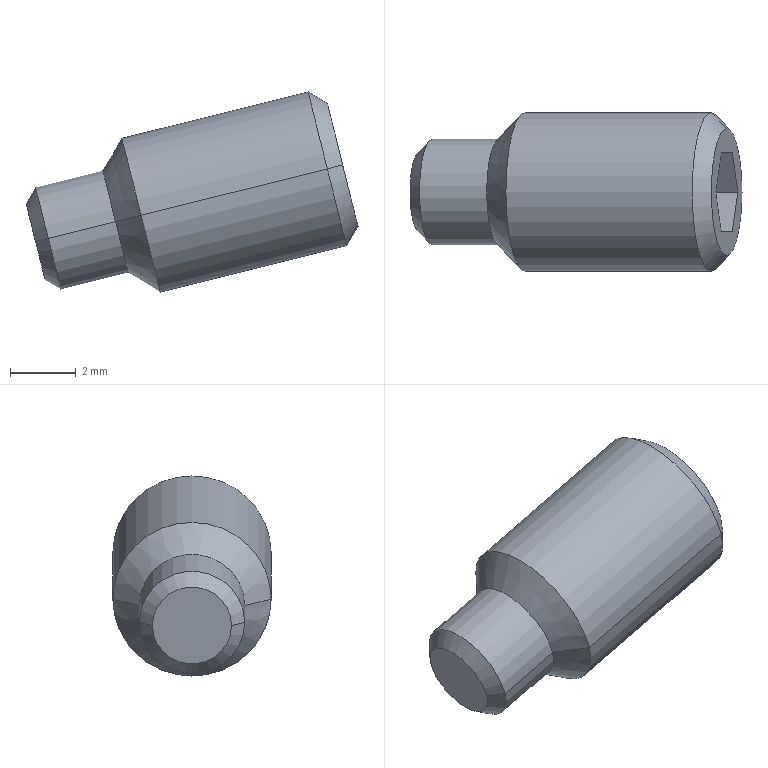Part | SolidWorks | features BaseBody 1 | 1 solid | 19 faces | box 10.07 x 4.8 x 6.065 mm | volume 127.97 mm3 | plane 9 | cone 6 | cylinder 4 | commonest cylinder face diameters 3.2 x2 4.8 x2
STEP:
#1=CARTESIAN_POINT('',(-2069.33,548.067,-1553.025));
#2=VERTEX_POINT('',#1);
#3=CARTESIAN_POINT('',(-2069.718,548.467,-1553.121));
#4=VERTEX_POINT('',#3);
#5=CARTESIAN_POINT('',(-2069.33,548.067,-1553.025));
#6=DIRECTION('',(-0.6861,0.7071,-0.1711));
#7=VECTOR('',#6,1000.);
#8=LINE('',#5,#7);
#9=EDGE_CURVE('',#2,#4,#8,.T.);
#10=ORIENTED_EDGE('',*,*,#9,.T.);
#11=CARTESIAN_POINT('',(-2069.718,550.867,-1553.121));
#12=VERTEX_POINT('',#11);
#13=CARTESIAN_POINT('',(-2069.718,549.667,-1553.121));
#14=DIRECTION('',(-0.9703,0.,-0.2419));
#15=DIRECTION('',(0.,1.,0.));
#16=AXIS2_PLACEMENT_3D('',#13,#14,#15);
#17=CIRCLE('',#16,1.2);
#18=EDGE_CURVE('',#12,#4,#17,.T.);
#19=ORIENTED_EDGE('',*,*,#18,.F.);
#20=CARTESIAN_POINT('',(-2069.33,551.267,-1553.025));
#21=VERTEX_POINT('',#20);
#22=CARTESIAN_POINT('',(-2069.718,550.867,-1553.121));
#23=DIRECTION('',(0.6861,0.7071,0.1711));
#24=VECTOR('',#23,1000.);
#25=LINE('',#22,#24);
#26=EDGE_CURVE('',#12,#21,#25,.T.);
#27=ORIENTED_EDGE('',*,*,#26,.T.);
#28=CARTESIAN_POINT('',(-2069.33,549.667,-1553.025));
#29=DIRECTION('',(0.9703,0.,0.2419));
#30=DIRECTION('',(0.,-1.,0.));
#31=AXIS2_PLACEMENT_3D('',#28,#29,#30);
#32=CIRCLE('',#31,1.6);
#33=EDGE_CURVE('',#2,#21,#32,.T.);
#34=ORIENTED_EDGE('',*,*,#33,.F.);
#35=EDGE_LOOP('',(#10,#19,#27,#34));
#36=FACE_OUTER_BOUND('',#35,.T.);
#37=CARTESIAN_POINT('',(-2069.738,549.667,-1553.126));
#38=DIRECTION('',(0.9703,0.,0.2419));
#39=DIRECTION('',(-0.02108,-0.9962,0.08457));
#40=AXIS2_PLACEMENT_3D('',#37,#38,#39);
#41=CONICAL_SURFACE('',#40,1.18,0.7854);
#42=ADVANCED_FACE('',(#36),#41,.T.);
#43=CARTESIAN_POINT('',(-2067.293,548.067,-1552.517));
#44=VERTEX_POINT('',#43);
#45=CARTESIAN_POINT('',(-2067.293,548.067,-1552.517));
#46=DIRECTION('',(-0.9703,0.,-0.2419));
#47=VECTOR('',#46,1000.);
#48=LINE('',#45,#47);
#49=EDGE_CURVE('',#44,#2,#48,.T.);
#50=ORIENTED_EDGE('',*,*,#49,.T.);
#51=ORIENTED_EDGE('',*,*,#33,.T.);
#52=CARTESIAN_POINT('',(-2067.293,551.267,-1552.517));
#53=VERTEX_POINT('',#52);
#54=CARTESIAN_POINT('',(-2069.33,551.267,-1553.025));
#55=DIRECTION('',(0.9703,0.,0.2419));
#56=VECTOR('',#55,1000.);
#57=LINE('',#54,#56);
#58=EDGE_CURVE('',#21,#53,#57,.T.);
#59=ORIENTED_EDGE('',*,*,#58,.T.);
#60=CARTESIAN_POINT('',(-2067.293,549.667,-1552.517));
#61=DIRECTION('',(0.9703,0.,0.2419));
#62=DIRECTION('',(0.,-1.,0.));
#63=AXIS2_PLACEMENT_3D('',#60,#61,#62);
#64=CIRCLE('',#63,1.6);
#65=EDGE_CURVE('',#44,#53,#64,.T.);
#66=ORIENTED_EDGE('',*,*,#65,.F.);
#67=EDGE_LOOP('',(#50,#51,#59,#66));
#68=FACE_OUTER_BOUND('',#67,.T.);
#69=CARTESIAN_POINT('',(-2067.191,549.667,-1552.491));
#70=DIRECTION('',(0.9703,0.,0.2419));
#71=DIRECTION('',(-0.02108,-0.9962,0.08457));
#72=AXIS2_PLACEMENT_3D('',#69,#70,#71);
#73=CYLINDRICAL_SURFACE('',#72,1.6);
#74=ADVANCED_FACE('',(#68),#73,.T.);
#75=CARTESIAN_POINT('',(-2066.517,547.267,-1552.323));
#76=VERTEX_POINT('',#75);
#77=CARTESIAN_POINT('',(-2066.517,547.267,-1552.323));
#78=DIRECTION('',(-0.6861,0.7071,-0.1711));
#79=VECTOR('',#78,1000.);
#80=LINE('',#77,#79);
#81=EDGE_CURVE('',#76,#44,#80,.T.);
#82=ORIENTED_EDGE('',*,*,#81,.T.);
#83=ORIENTED_EDGE('',*,*,#65,.T.);
#84=CARTESIAN_POINT('',(-2066.517,552.067,-1552.323));
#85=VERTEX_POINT('',#84);
#86=CARTESIAN_POINT('',(-2067.293,551.267,-1552.517));
#87=DIRECTION('',(0.6861,0.7071,0.1711));
#88=VECTOR('',#87,1000.);
#89=LINE('',#86,#88);
#90=EDGE_CURVE('',#53,#85,#89,.T.);
#91=ORIENTED_EDGE('',*,*,#90,.T.);
#92=CARTESIAN_POINT('',(-2066.517,549.667,-1552.323));
#93=DIRECTION('',(0.9703,0.,0.2419));
#94=DIRECTION('',(0.,-1.,0.));
#95=AXIS2_PLACEMENT_3D('',#92,#93,#94);
#96=CIRCLE('',#95,2.4);
#97=EDGE_CURVE('',#76,#85,#96,.T.);
#98=ORIENTED_EDGE('',*,*,#97,.F.);
#99=EDGE_LOOP('',(#82,#83,#91,#98));
#100=FACE_OUTER_BOUND('',#99,.T.);
#101=CARTESIAN_POINT('',(-2067.332,549.667,-1552.526));
#102=DIRECTION('',(0.9703,0.,0.2419));
#103=DIRECTION('',(-0.02108,-0.9962,0.08457));
#104=AXIS2_PLACEMENT_3D('',#101,#102,#103);
#105=CONICAL_SURFACE('',#104,1.56,0.7854);
#106=ADVANCED_FACE('',(#100),#105,.T.);
#107=CARTESIAN_POINT('',(-2060.869,547.267,-1550.915));
#108=VERTEX_POINT('',#107);
#109=CARTESIAN_POINT('',(-2060.404,547.747,-1550.799));
#110=VERTEX_POINT('',#109);
#111=CARTESIAN_POINT('',(-2060.869,547.267,-1550.915));
#112=DIRECTION('',(0.6861,0.7071,0.1711));
#113=VECTOR('',#112,1000.);
#114=LINE('',#111,#113);
#115=EDGE_CURVE('',#108,#110,#114,.T.);
#116=ORIENTED_EDGE('',*,*,#115,.T.);
#117=CARTESIAN_POINT('',(-2060.404,551.587,-1550.799));
#118=VERTEX_POINT('',#117);
#119=CARTESIAN_POINT('',(-2060.404,549.667,-1550.799));
#120=DIRECTION('',(0.9703,0.,0.2419));
#121=DIRECTION('',(0.,1.,0.));
#122=AXIS2_PLACEMENT_3D('',#119,#120,#121);
#123=CIRCLE('',#122,1.92);
#124=EDGE_CURVE('',#118,#110,#123,.T.);
#125=ORIENTED_EDGE('',*,*,#124,.F.);
#126=CARTESIAN_POINT('',(-2060.869,552.067,-1550.915));
#127=VERTEX_POINT('',#126);
#128=CARTESIAN_POINT('',(-2060.404,551.587,-1550.799));
#129=DIRECTION('',(-0.6861,0.7071,-0.1711));
#130=VECTOR('',#129,1000.);
#131=LINE('',#128,#130);
#132=EDGE_CURVE('',#118,#127,#131,.T.);
#133=ORIENTED_EDGE('',*,*,#132,.T.);
#134=CARTESIAN_POINT('',(-2060.869,549.667,-1550.915));
#135=DIRECTION('',(-0.9703,0.,-0.2419));
#136=DIRECTION('',(0.,-1.,0.));
#137=AXIS2_PLACEMENT_3D('',#134,#135,#136);
#138=CIRCLE('',#137,2.4);
#139=EDGE_CURVE('',#108,#127,#138,.T.);
#140=ORIENTED_EDGE('',*,*,#139,.F.);
#141=EDGE_LOOP('',(#116,#125,#133,#140));
#142=FACE_OUTER_BOUND('',#141,.T.);
#143=CARTESIAN_POINT('',(-2060.38,549.667,-1550.793));
#144=DIRECTION('',(-0.9703,0.,-0.2419));
#145=DIRECTION('',(0.02108,-0.9962,-0.08457));
#146=AXIS2_PLACEMENT_3D('',#143,#144,#145);
#147=CONICAL_SURFACE('',#146,1.896,0.7854);
#148=ADVANCED_FACE('',(#142),#147,.T.);
#149=CARTESIAN_POINT('',(-2066.517,552.067,-1552.323));
#150=DIRECTION('',(0.9703,0.,0.2419));
#151=VECTOR('',#150,1000.);
#152=LINE('',#149,#151);
#153=EDGE_CURVE('',#85,#127,#152,.T.);
#154=ORIENTED_EDGE('',*,*,#153,.T.);
#155=CARTESIAN_POINT('',(-2060.869,549.667,-1550.915));
#156=DIRECTION('',(-0.9703,0.,-0.2419));
#157=DIRECTION('',(0.,1.,0.));
#158=AXIS2_PLACEMENT_3D('',#155,#156,#157);
#159=CIRCLE('',#158,2.4);
#160=EDGE_CURVE('',#127,#108,#159,.T.);
#161=ORIENTED_EDGE('',*,*,#160,.T.);
#162=CARTESIAN_POINT('',(-2060.869,547.267,-1550.915));
#163=DIRECTION('',(-0.9703,0.,-0.2419));
#164=VECTOR('',#163,1000.);
#165=LINE('',#162,#164);
#166=EDGE_CURVE('',#108,#76,#165,.T.);
#167=ORIENTED_EDGE('',*,*,#166,.T.);
#168=ORIENTED_EDGE('',*,*,#97,.T.);
#169=EDGE_LOOP('',(#154,#161,#167,#168));
#170=FACE_OUTER_BOUND('',#169,.T.);
#171=CARTESIAN_POINT('',(-2066.799,549.667,-1552.393));
#172=DIRECTION('',(-0.9703,0.,-0.2419));
#173=DIRECTION('',(-0.02108,0.9962,0.08457));
#174=AXIS2_PLACEMENT_3D('',#171,#172,#173);
#175=CYLINDRICAL_SURFACE('',#174,2.4);
#176=ADVANCED_FACE('',(#170),#175,.T.);
#177=CARTESIAN_POINT('',(-2062.953,550.867,-1552.149));
#178=VERTEX_POINT('',#177);
#179=CARTESIAN_POINT('',(-2063.288,550.867,-1550.804));
#180=VERTEX_POINT('',#179);
#181=CARTESIAN_POINT('',(-2062.953,550.867,-1552.149));
#182=DIRECTION('',(-0.2419,0.,0.9703));
#183=VECTOR('',#182,1000.);
#184=LINE('',#181,#183);
#185=EDGE_CURVE('',#178,#180,#184,.T.);
#186=ORIENTED_EDGE('',*,*,#185,.T.);
#187=CARTESIAN_POINT('',(-2063.456,549.667,-1550.132));
#188=VERTEX_POINT('',#187);
#189=CARTESIAN_POINT('',(-2063.288,550.867,-1550.804));
#190=DIRECTION('',(-0.121,-0.866,0.4851));
#191=VECTOR('',#190,1000.);
#192=LINE('',#189,#191);
#193=EDGE_CURVE('',#180,#188,#192,.T.);
#194=ORIENTED_EDGE('',*,*,#193,.T.);
#195=CARTESIAN_POINT('',(-2063.288,548.467,-1550.804));
#196=VERTEX_POINT('',#195);
#197=CARTESIAN_POINT('',(-2063.456,549.667,-1550.132));
#198=DIRECTION('',(0.121,-0.866,-0.4851));
#199=VECTOR('',#198,1000.);
#200=LINE('',#197,#199);
#201=EDGE_CURVE('',#188,#196,#200,.T.);
#202=ORIENTED_EDGE('',*,*,#201,.T.);
#203=CARTESIAN_POINT('',(-2062.953,548.467,-1552.149));
#204=VERTEX_POINT('',#203);
#205=CARTESIAN_POINT('',(-2063.288,548.467,-1550.804));
#206=DIRECTION('',(0.2419,0.,-0.9703));
#207=VECTOR('',#206,1000.);
#208=LINE('',#205,#207);
#209=EDGE_CURVE('',#196,#204,#208,.T.);
#210=ORIENTED_EDGE('',*,*,#209,.T.);
#211=CARTESIAN_POINT('',(-2062.785,549.667,-1552.821));
#212=VERTEX_POINT('',#211);
#213=CARTESIAN_POINT('',(-2062.953,548.467,-1552.149));
#214=DIRECTION('',(0.121,0.866,-0.4851));
#215=VECTOR('',#214,1000.);
#216=LINE('',#213,#215);
#217=EDGE_CURVE('',#204,#212,#216,.T.);
#218=ORIENTED_EDGE('',*,*,#217,.T.);
#219=CARTESIAN_POINT('',(-2062.785,549.667,-1552.821));
#220=DIRECTION('',(-0.121,0.866,0.4851));
#221=VECTOR('',#220,1000.);
#222=LINE('',#219,#221);
#223=EDGE_CURVE('',#212,#178,#222,.T.);
#224=ORIENTED_EDGE('',*,*,#223,.T.);
#225=EDGE_LOOP('',(#186,#194,#202,#210,#218,#224));
#226=FACE_OUTER_BOUND('',#225,.T.);
#227=CARTESIAN_POINT('',(-2062.752,548.328,-1552.955));
#228=DIRECTION('',(0.9703,0.,0.2419));
#229=DIRECTION('',(0.,-1.,0.));
#230=AXIS2_PLACEMENT_3D('',#227,#228,#229);
#231=PLANE('',#230);
#232=ADVANCED_FACE('',(#226),#231,.T.);
#233=CARTESIAN_POINT('',(-2060.068,549.667,-1552.143));
#234=VERTEX_POINT('',#233);
#235=CARTESIAN_POINT('',(-2060.236,550.867,-1551.471));
#236=VERTEX_POINT('',#235);
#237=CARTESIAN_POINT('',(-2060.068,549.667,-1552.143));
#238=DIRECTION('',(-0.121,0.866,0.4851));
#239=VECTOR('',#238,1000.);
#240=LINE('',#237,#239);
#241=EDGE_CURVE('',#234,#236,#240,.T.);
#242=ORIENTED_EDGE('',*,*,#241,.T.);
#243=CARTESIAN_POINT('',(-2062.953,550.867,-1552.149));
#244=DIRECTION('',(0.9703,0.,0.2419));
#245=VECTOR('',#244,1000.);
#246=LINE('',#243,#245);
#247=EDGE_CURVE('',#178,#236,#246,.T.);
#248=ORIENTED_EDGE('',*,*,#247,.F.);
#249=ORIENTED_EDGE('',*,*,#223,.F.);
#250=CARTESIAN_POINT('',(-2062.785,549.667,-1552.821));
#251=DIRECTION('',(0.9703,0.,0.2419));
#252=VECTOR('',#251,1000.);
#253=LINE('',#250,#252);
#254=EDGE_CURVE('',#212,#234,#253,.T.);
#255=ORIENTED_EDGE('',*,*,#254,.T.);
#256=EDGE_LOOP('',(#242,#248,#249,#255));
#257=FACE_OUTER_BOUND('',#256,.T.);
#258=CARTESIAN_POINT('',(-2059.916,549.545,-1552.177));
#259=DIRECTION('',(-0.2095,-0.5,0.8403));
#260=DIRECTION('',(-0.9223,0.3865,0.));
#261=AXIS2_PLACEMENT_3D('',#258,#259,#260);
#262=PLANE('',#261);
#263=ADVANCED_FACE('',(#257),#262,.T.);
#264=CARTESIAN_POINT('',(-2060.236,548.467,-1551.471));
#265=VERTEX_POINT('',#264);
#266=CARTESIAN_POINT('',(-2060.236,548.467,-1551.471));
#267=DIRECTION('',(0.121,0.866,-0.4851));
#268=VECTOR('',#267,1000.);
#269=LINE('',#266,#268);
#270=EDGE_CURVE('',#265,#234,#269,.T.);
#271=ORIENTED_EDGE('',*,*,#270,.T.);
#272=ORIENTED_EDGE('',*,*,#254,.F.);
#273=ORIENTED_EDGE('',*,*,#217,.F.);
#274=CARTESIAN_POINT('',(-2062.953,548.467,-1552.149));
#275=DIRECTION('',(0.9703,0.,0.2419));
#276=VECTOR('',#275,1000.);
#277=LINE('',#274,#276);
#278=EDGE_CURVE('',#204,#265,#277,.T.);
#279=ORIENTED_EDGE('',*,*,#278,.T.);
#280=EDGE_LOOP('',(#271,#272,#273,#279));
#281=FACE_OUTER_BOUND('',#280,.T.);
#282=CARTESIAN_POINT('',(-2060.117,548.345,-1551.369));
#283=DIRECTION('',(-0.2095,0.5,0.8403));
#284=DIRECTION('',(0.9223,0.3865,0.));
#285=AXIS2_PLACEMENT_3D('',#282,#283,#284);
#286=PLANE('',#285);
#287=ADVANCED_FACE('',(#281),#286,.T.);
#288=CARTESIAN_POINT('',(-2060.571,548.467,-1550.127));
#289=VERTEX_POINT('',#288);
#290=CARTESIAN_POINT('',(-2060.571,548.467,-1550.127));
#291=DIRECTION('',(0.2419,0.,-0.9703));
#292=VECTOR('',#291,1000.);
#293=LINE('',#290,#292);
#294=EDGE_CURVE('',#289,#265,#293,.T.);
#295=ORIENTED_EDGE('',*,*,#294,.T.);
#296=ORIENTED_EDGE('',*,*,#278,.F.);
#297=ORIENTED_EDGE('',*,*,#209,.F.);
#298=CARTESIAN_POINT('',(-2063.288,548.467,-1550.804));
#299=DIRECTION('',(0.9703,0.,0.2419));
#300=VECTOR('',#299,1000.);
#301=LINE('',#298,#300);
#302=EDGE_CURVE('',#196,#289,#301,.T.);
#303=ORIENTED_EDGE('',*,*,#302,.T.);
#304=EDGE_LOOP('',(#295,#296,#297,#303));
#305=FACE_OUTER_BOUND('',#304,.T.);
#306=CARTESIAN_POINT('',(-2060.469,548.467,-1549.957));
#307=DIRECTION('',(0.,1.,0.));
#308=DIRECTION('',(1.,0.,0.));
#309=AXIS2_PLACEMENT_3D('',#306,#307,#308);
#310=PLANE('',#309);
#311=ADVANCED_FACE('',(#305),#310,.T.);
#312=CARTESIAN_POINT('',(-2060.739,549.667,-1549.454));
#313=VERTEX_POINT('',#312);
#314=CARTESIAN_POINT('',(-2060.739,549.667,-1549.454));
#315=DIRECTION('',(0.121,-0.866,-0.4851));
#316=VECTOR('',#315,1000.);
#317=LINE('',#314,#316);
#318=EDGE_CURVE('',#313,#289,#317,.T.);
#319=ORIENTED_EDGE('',*,*,#318,.T.);
#320=ORIENTED_EDGE('',*,*,#302,.F.);
#321=ORIENTED_EDGE('',*,*,#201,.F.);
#322=CARTESIAN_POINT('',(-2063.456,549.667,-1550.132));
#323=DIRECTION('',(0.9703,0.,0.2419));
#324=VECTOR('',#323,1000.);
#325=LINE('',#322,#324);
#326=EDGE_CURVE('',#188,#313,#325,.T.);
#327=ORIENTED_EDGE('',*,*,#326,.T.);
#328=EDGE_LOOP('',(#319,#320,#321,#327));
#329=FACE_OUTER_BOUND('',#328,.T.);
#330=CARTESIAN_POINT('',(-2060.62,549.788,-1549.353));
#331=DIRECTION('',(0.2095,0.5,-0.8403));
#332=DIRECTION('',(-0.9703,0.,-0.2419));
#333=AXIS2_PLACEMENT_3D('',#330,#331,#332);
#334=PLANE('',#333);
#335=ADVANCED_FACE('',(#329),#334,.T.);
#336=CARTESIAN_POINT('',(-2060.571,550.867,-1550.127));
#337=VERTEX_POINT('',#336);
#338=CARTESIAN_POINT('',(-2060.571,550.867,-1550.127));
#339=DIRECTION('',(-0.121,-0.866,0.4851));
#340=VECTOR('',#339,1000.);
#341=LINE('',#338,#340);
#342=EDGE_CURVE('',#337,#313,#341,.T.);
#343=ORIENTED_EDGE('',*,*,#342,.T.);
#344=ORIENTED_EDGE('',*,*,#326,.F.);
#345=ORIENTED_EDGE('',*,*,#193,.F.);
#346=CARTESIAN_POINT('',(-2063.288,550.867,-1550.804));
#347=DIRECTION('',(0.9703,0.,0.2419));
#348=VECTOR('',#347,1000.);
#349=LINE('',#346,#348);
#350=EDGE_CURVE('',#180,#337,#349,.T.);
#351=ORIENTED_EDGE('',*,*,#350,.T.);
#352=EDGE_LOOP('',(#343,#344,#345,#351));
#353=FACE_OUTER_BOUND('',#352,.T.);
#354=CARTESIAN_POINT('',(-2060.418,550.988,-1550.161));
#355=DIRECTION('',(0.2095,-0.5,-0.8403));
#356=DIRECTION('',(0.,-0.8594,0.5113));
#357=AXIS2_PLACEMENT_3D('',#354,#355,#356);
#358=PLANE('',#357);
#359=ADVANCED_FACE('',(#353),#358,.T.);
#360=CARTESIAN_POINT('',(-2060.236,550.867,-1551.471));
#361=DIRECTION('',(-0.2419,0.,0.9703));
#362=VECTOR('',#361,1000.);
#363=LINE('',#360,#362);
#364=EDGE_CURVE('',#236,#337,#363,.T.);
#365=ORIENTED_EDGE('',*,*,#364,.T.);
#366=ORIENTED_EDGE('',*,*,#350,.F.);
#367=ORIENTED_EDGE('',*,*,#185,.F.);
#368=ORIENTED_EDGE('',*,*,#247,.T.);
#369=EDGE_LOOP('',(#365,#366,#367,#368));
#370=FACE_OUTER_BOUND('',#369,.T.);
#371=CARTESIAN_POINT('',(-2060.469,550.867,-1549.957));
#372=DIRECTION('',(0.,-1.,0.));
#373=DIRECTION('',(0.,0.,-1.));
#374=AXIS2_PLACEMENT_3D('',#371,#372,#373);
#375=PLANE('',#374);
#376=ADVANCED_FACE('',(#370),#375,.T.);
#377=ORIENTED_EDGE('',*,*,#18,.T.);
#378=CARTESIAN_POINT('',(-2069.718,549.667,-1553.121));
#379=DIRECTION('',(-0.9703,0.,-0.2419));
#380=DIRECTION('',(0.,-1.,0.));
#381=AXIS2_PLACEMENT_3D('',#378,#379,#380);
#382=CIRCLE('',#381,1.2);
#383=EDGE_CURVE('',#4,#12,#382,.T.);
#384=ORIENTED_EDGE('',*,*,#383,.T.);
#385=EDGE_LOOP('',(#377,#384));
#386=FACE_OUTER_BOUND('',#385,.T.);
#387=CARTESIAN_POINT('',(-2069.402,550.987,-1554.39));
#388=DIRECTION('',(-0.9703,0.,-0.2419));
#389=DIRECTION('',(-0.2419,0.,0.9703));
#390=AXIS2_PLACEMENT_3D('',#387,#388,#389);
#391=PLANE('',#390);
#392=ADVANCED_FACE('',(#386),#391,.T.);
#393=ORIENTED_EDGE('',*,*,#26,.F.);
#394=ORIENTED_EDGE('',*,*,#383,.F.);
#395=ORIENTED_EDGE('',*,*,#9,.F.);
#396=CARTESIAN_POINT('',(-2069.33,549.667,-1553.025));
#397=DIRECTION('',(0.9703,0.,0.2419));
#398=DIRECTION('',(0.,1.,0.));
#399=AXIS2_PLACEMENT_3D('',#396,#397,#398);
#400=CIRCLE('',#399,1.6);
#401=EDGE_CURVE('',#21,#2,#400,.T.);
#402=ORIENTED_EDGE('',*,*,#401,.F.);
#403=EDGE_LOOP('',(#393,#394,#395,#402));
#404=FACE_OUTER_BOUND('',#403,.T.);
#405=CARTESIAN_POINT('',(-2069.738,549.667,-1553.126));
#406=DIRECTION('',(0.9703,0.,0.2419));
#407=DIRECTION('',(0.02108,0.9962,-0.08457));
#408=AXIS2_PLACEMENT_3D('',#405,#406,#407);
#409=CONICAL_SURFACE('',#408,1.18,0.7854);
#410=ADVANCED_FACE('',(#404),#409,.T.);
#411=ORIENTED_EDGE('',*,*,#58,.F.);
#412=ORIENTED_EDGE('',*,*,#401,.T.);
#413=ORIENTED_EDGE('',*,*,#49,.F.);
#414=CARTESIAN_POINT('',(-2067.293,549.667,-1552.517));
#415=DIRECTION('',(0.9703,0.,0.2419));
#416=DIRECTION('',(0.,1.,0.));
#417=AXIS2_PLACEMENT_3D('',#414,#415,#416);
#418=CIRCLE('',#417,1.6);
#419=EDGE_CURVE('',#53,#44,#418,.T.);
#420=ORIENTED_EDGE('',*,*,#419,.F.);
#421=EDGE_LOOP('',(#411,#412,#413,#420));
#422=FACE_OUTER_BOUND('',#421,.T.);
#423=CARTESIAN_POINT('',(-2067.191,549.667,-1552.491));
#424=DIRECTION('',(0.9703,0.,0.2419));
#425=DIRECTION('',(0.02108,0.9962,-0.08457));
#426=AXIS2_PLACEMENT_3D('',#423,#424,#425);
#427=CYLINDRICAL_SURFACE('',#426,1.6);
#428=ADVANCED_FACE('',(#422),#427,.T.);
#429=ORIENTED_EDGE('',*,*,#90,.F.);
#430=ORIENTED_EDGE('',*,*,#419,.T.);
#431=ORIENTED_EDGE('',*,*,#81,.F.);
#432=CARTESIAN_POINT('',(-2066.517,549.667,-1552.323));
#433=DIRECTION('',(0.9703,0.,0.2419));
#434=DIRECTION('',(0.,1.,0.));
#435=AXIS2_PLACEMENT_3D('',#432,#433,#434);
#436=CIRCLE('',#435,2.4);
#437=EDGE_CURVE('',#85,#76,#436,.T.);
#438=ORIENTED_EDGE('',*,*,#437,.F.);
#439=EDGE_LOOP('',(#429,#430,#431,#438));
#440=FACE_OUTER_BOUND('',#439,.T.);
#441=CARTESIAN_POINT('',(-2067.332,549.667,-1552.526));
#442=DIRECTION('',(0.9703,0.,0.2419));
#443=DIRECTION('',(0.02108,0.9962,-0.08457));
#444=AXIS2_PLACEMENT_3D('',#441,#442,#443);
#445=CONICAL_SURFACE('',#444,1.56,0.7854);
#446=ADVANCED_FACE('',(#440),#445,.T.);
#447=ORIENTED_EDGE('',*,*,#132,.F.);
#448=CARTESIAN_POINT('',(-2060.404,549.667,-1550.799));
#449=DIRECTION('',(0.9703,0.,0.2419));
#450=DIRECTION('',(0.,-1.,0.));
#451=AXIS2_PLACEMENT_3D('',#448,#449,#450);
#452=CIRCLE('',#451,1.92);
#453=EDGE_CURVE('',#110,#118,#452,.T.);
#454=ORIENTED_EDGE('',*,*,#453,.F.);
#455=ORIENTED_EDGE('',*,*,#115,.F.);
#456=ORIENTED_EDGE('',*,*,#160,.F.);
#457=EDGE_LOOP('',(#447,#454,#455,#456));
#458=FACE_OUTER_BOUND('',#457,.T.);
#459=CARTESIAN_POINT('',(-2060.38,549.667,-1550.793));
#460=DIRECTION('',(-0.9703,0.,-0.2419));
#461=DIRECTION('',(-0.02108,0.9962,0.08457));
#462=AXIS2_PLACEMENT_3D('',#459,#460,#461);
#463=CONICAL_SURFACE('',#462,1.896,0.7854);
#464=ADVANCED_FACE('',(#458),#463,.T.);
#465=ORIENTED_EDGE('',*,*,#364,.F.);
#466=ORIENTED_EDGE('',*,*,#241,.F.);
#467=ORIENTED_EDGE('',*,*,#270,.F.);
#468=ORIENTED_EDGE('',*,*,#294,.F.);
#469=ORIENTED_EDGE('',*,*,#318,.F.);
#470=ORIENTED_EDGE('',*,*,#342,.F.);
#471=EDGE_LOOP('',(#465,#466,#467,#468,#469,#470));
#472=FACE_BOUND('',#471,.T.);
#473=ORIENTED_EDGE('',*,*,#453,.T.);
#474=ORIENTED_EDGE('',*,*,#124,.T.);
#475=EDGE_LOOP('',(#473,#474));
#476=FACE_OUTER_BOUND('',#475,.T.);
#477=CARTESIAN_POINT('',(-2059.897,547.555,-1552.829));
#478=DIRECTION('',(0.9703,0.,0.2419));
#479=DIRECTION('',(0.,-1.,0.));
#480=AXIS2_PLACEMENT_3D('',#477,#478,#479);
#481=PLANE('',#480);
#482=ADVANCED_FACE('',(#472,#476),#481,.T.);
#483=ORIENTED_EDGE('',*,*,#166,.F.);
#484=ORIENTED_EDGE('',*,*,#139,.T.);
#485=ORIENTED_EDGE('',*,*,#153,.F.);
#486=ORIENTED_EDGE('',*,*,#437,.T.);
#487=EDGE_LOOP('',(#483,#484,#485,#486));
#488=FACE_OUTER_BOUND('',#487,.T.);
#489=CARTESIAN_POINT('',(-2066.799,549.667,-1552.393));
#490=DIRECTION('',(-0.9703,0.,-0.2419));
#491=DIRECTION('',(0.02108,-0.9962,-0.08457));
#492=AXIS2_PLACEMENT_3D('',#489,#490,#491);
#493=CYLINDRICAL_SURFACE('',#492,2.4);
#494=ADVANCED_FACE('',(#488),#493,.T.);
#495=CLOSED_SHELL('',(#42,#74,#106,#148,#176,#232,#263,#287,#311,#335,#359,#376,#392,#410,#428,#446,#464,#482,#494));
#496=MANIFOLD_SOLID_BREP('',#495);
#497=CARTESIAN_POINT('',(0.,0.,0.));
#498=DIRECTION('',(0.,0.,1.));
#499=DIRECTION('',(1.,0.,0.));
#500=AXIS2_PLACEMENT_3D('',#497,#498,#499);
#501=(LENGTH_UNIT()NAMED_UNIT(*)SI_UNIT(.MILLI.,.METRE.));
#502=UNCERTAINTY_MEASURE_WITH_UNIT(LENGTH_MEASURE(0.00001),#501,'','');
#503=(NAMED_UNIT(*)PLANE_ANGLE_UNIT()SI_UNIT($,.RADIAN.));
#504=(NAMED_UNIT(*)SI_UNIT($,.STERADIAN.)SOLID_ANGLE_UNIT());
#505=(GEOMETRIC_REPRESENTATION_CONTEXT(3)GLOBAL_UNCERTAINTY_ASSIGNED_CONTEXT((#502))GLOBAL_UNIT_ASSIGNED_CONTEXT((#501,#503,#504))REPRESENTATION_CONTEXT('',''));
#506=ADVANCED_BREP_SHAPE_REPRESENTATION('',(#496,#500),#505);